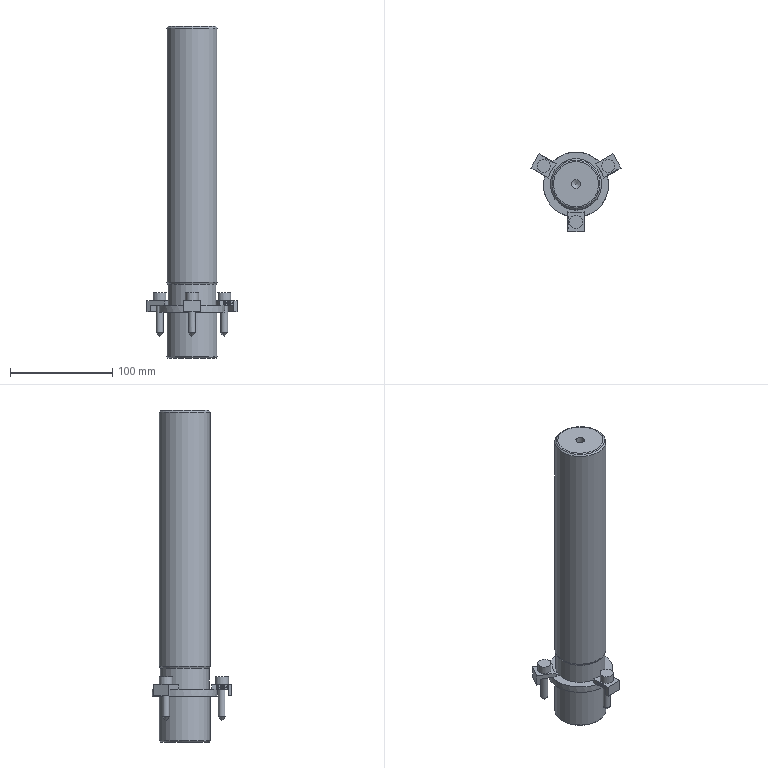Part | STEP file | lll_id614_x_t | 1 solid | 184 faces | box 88.144 x 78.2 x 325 mm | volume 648691 mm3 | plane 106 | other 57 | cylinder 12 | cone 8 | torus 1 | commonest cylinder face diameters 6.8 x3 13 x3 50 x2 8.5 x1 10.5 x1 48 x1